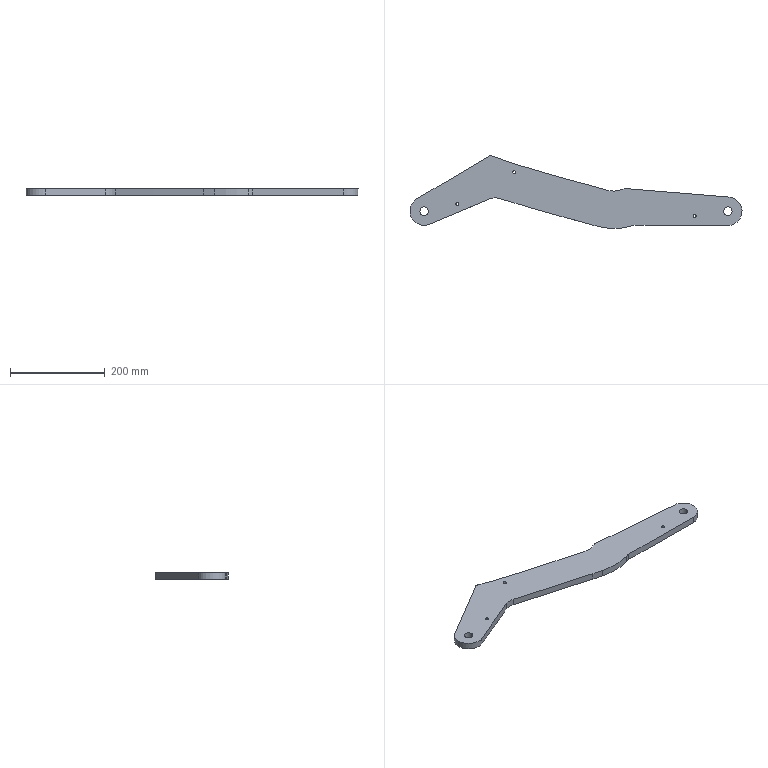NC program | NX | posted with a generic post | part box 700 x 153.975 x 14 mm
Lines 1 to 967 of 6173:
N10 G17 G21 G94 G90
(CAVITY_MILL , TOOL : D20R0)
N12 T00 M6
N14 G54
N16 G17 G0 G90 X361.565 Y64.401 S4500 M3
N18 G43 Z117. H0
N20 Z19.
N22 G94 G1 X361.412 Y64.442 Z18.994 F3500.
N24 X361.381 Y64.45 Z18.993
N26 X361.29 Y64.475 Z18.99
N28 X361.044 Y64.541 Z18.981
N30 X360.012 Y64.819 Z18.944
N32 X359.496 Y64.958 Z18.925
N34 X358.464 Y65.237 Z18.888
N36 X357.948 Y65.376 Z18.869
N38 X357.329 Y65.543 Z18.847
N40 X357.174 Y65.585 Z18.841
N42 X357.019 Y65.628 Z18.836
N44 X356.922 Y65.653 Z18.832
N46 X356.859 Y65.67 Z18.83
N48 X356.855 Y65.671
N50 X356.85 Z18.829
N52 X356.846 Y65.673
N54 X356.842 Y65.674
N56 X356.659 Y65.725 Z18.823
N58 X356.572 Y65.749 Z18.819
N60 X356.486 Y65.772 Z18.816
N62 X356.4 Y65.796 Z18.813
N64 X355.368 Y66.075 Z18.776
N66 X354.852 Y66.215 Z18.757
N68 X354.466 Y66.321 Z18.743
N70 X354.272 Y66.374 Z18.736
N72 X354.079 Y66.426 Z18.729
N74 X353.866 Y66.484 Z18.721
N76 X353.772 Y66.509 Z18.718
N78 X353.725 Y66.522 Z18.716
N80 X351.154 Y67.22 Z18.623
N82 X351.132 Y67.226
N84 X351.117 Y67.23 Z18.622
N86 X345.426 Y68.777 Z18.416
N88 X339.758 Y70.326 Z18.211
N90 X328.471 Y73.421 Z17.802
N92 X317.261 Y76.52 Z17.396
N94 X311.678 Y78.068 Z17.194
N96 X300.575 Y81.165 Z16.791
N98 X295.05 Y82.714 Z16.591
N100 X289.54 Y84.263 Z16.391
N102 X284.042 Y85.811 Z16.191
N104 X278.766 Y87.306 Z16.
N106 X273.108 Y88.909
N108 X267.673 Y90.457
N110 X262.251 Y92.006
N112 X256.852 Y93.554
N114 X251.475 Y95.103
N116 X246.109 Y96.648
N118 X240.773 Y98.171
N120 X235.47 Y99.72
N122 X229.46 Y101.483
N124 X219.734 Y104.365
N126 X213.98 Y106.087
N128 X209.427 Y107.462
N130 X203.145 Y109.375
N132 X199.3 Y110.56
N134 X194.321 Y112.108
N136 X193.857 Y112.254
N138 X189.412 Y113.657
N140 X187.666 Y114.211
N142 X181.474 Y116.211
N144 X176.83 Y117.745
N146 X173.735 Y118.785
N148 X170.627 Y119.85
N150 X169.091 Y120.382
N152 X166.204 Y121.399
N154 X164.448 Y122.029
N156 X161.936 Y122.947
N158 X159.805 Y123.74
N160 X157.815 Y124.495
N162 X155.162 Y125.531
N164 X153.891 Y126.044
N166 X152.067 Y126.791
N168 X150.187 Y127.592
N170 X148.972 Y128.117
N172 X147.426 Y128.798
N174 X146.629 Y129.213
N176 X146.618 Y129.217
N178 X145.876 Y129.432
N180 X144.329 Y129.881
N182 X144.326
N184 G3 X133.637 Y129.192 R18.085
N186 X130.388 Y127.613 R18.688
N188 G1 X-22.008 Y37.045
N190 G3 X-42.161 Y-8.75 R43.216
N192 X-4.312 Y-42.883 R43.059
N194 G1 X-4.079 Y-42.91
N196 X-4.075 Y-42.911
N198 X-2.758 Y-42.972
N200 X-1.21 Y-43.043
N202 X-1.208
N204 G3 X16.738 Y-39.674 R43.117
N206 G1 X16.798 Y-39.652
N208 X16.77 Y-39.595
N210 X16.742 Y-39.607
N212 G2 X4.084 Y-42.806 R43.
N214 X-21.987 Y36.954 R43.
N216 G1 X130.842 Y127.779
N218 G2 X147.304 Y128.786 R18.013
N220 G1 X148.863 Y128.099
N222 G3 X166.183 Y121.342 R260.503
N224 X195.387 Y111.711 R807.662
N226 X243.375 Y97.35 R2615.076
N228 X390.581 Y56.555 R6730.508
N230 X415.708 Y58.845 R36.87
N232 G1 X416.068 Y59.015
N234 G2 X425.196 Y60.668 R18.
N236 G1 X643.496 Y42.858
N238 G2 X644.084 Y-42.806 R43.
N240 X639.828 Y-43. R42.995
N242 G1 X639.792
N244 X639.789 Y-43.064
N246 X639.852 Y-43.06
N248 G3 X675.875 Y23.815 R43.064
N250 X644.312 Y42.88 R43.055
N252 G1 X644.311
N254 X642.762 Y43.007
N256 X426.043 Y60.659
N258 G3 X415.164 Y58.693 R19.291
N260 G1 X413.63 Y58.008
N262 X413.37 Y57.907
N264 X412.085 Y57.432
N266 X410.54 Y56.933
N268 X408.994 Y56.508
N270 X408.389 Y56.36
N272 X407.449 Y56.154
N274 X405.904 Y55.868
N276 X404.358 Y55.651
N278 X402.813 Y55.5
N280 X401.267 Y55.414
N282 X399.722 Y55.393
N284 X398.176 Y55.437
N286 X396.631 Y55.547
N288 X395.085 Y55.722
N290 X393.54 Y55.963
N292 X392.001 Y56.295
N294 X391.812 Y56.345
N296 X391.628 Y56.394
N298 X390.463 Y56.704
N300 X379.896 Y59.519
N302 X368.315 Y62.603
N304 X362.586 Y64.129
N306 X362.576 Y64.132
N308 X362.548 Y64.139
N310 X362.517 Y64.148
N312 X361.412 Y64.442
N314 X361.381 Y64.45
N316 X361.29 Y64.475
N318 X361.044 Y64.541
N320 X360.012 Y64.819
N322 X359.496 Y64.958
N324 X358.464 Y65.237
N326 X357.948 Y65.376
N328 X357.329 Y65.543
N330 X357.174 Y65.585
N332 X357.019 Y65.628
N334 X356.922 Y65.653
N336 X356.859 Y65.67
N338 X356.85 Y65.671
N340 X356.842 Y65.674
N342 X356.659 Y65.725
N344 X356.573 Y65.749
N346 X356.486 Y65.772
N348 X356.4 Y65.796
N350 X355.368 Y66.075
N352 X354.852 Y66.215
N354 X354.466 Y66.321
N356 X354.272 Y66.374
N358 X354.079 Y66.426
N360 X353.866 Y66.484
N362 X353.772 Y66.509
N364 X353.725 Y66.522
N366 X351.154 Y67.22
N368 X351.132 Y67.226
N370 X351.117 Y67.23
N372 X345.426 Y68.777
N374 X339.758 Y70.326
N376 X328.471 Y73.421
N378 X317.261 Y76.52
N380 X311.678 Y78.068
N382 X300.575 Y81.165
N384 X295.05 Y82.714
N386 X289.54 Y84.263
N388 X284.042 Y85.811
N390 X278.766 Y87.306
N392 Z19.
N394 G0 Z22.
N396 X361.565 Y64.401
N398 Z18.
N400 G1 X361.412 Y64.442 Z17.994
N402 X361.381 Y64.45 Z17.993
N404 X361.29 Y64.475 Z17.99
N406 X361.044 Y64.541 Z17.981
N408 X360.012 Y64.819 Z17.944
N410 X359.496 Y64.958 Z17.925
N412 X358.464 Y65.237 Z17.888
N414 X357.948 Y65.376 Z17.869
N416 X357.329 Y65.543 Z17.847
N418 X357.174 Y65.585 Z17.841
N420 X357.019 Y65.628 Z17.836
N422 X356.922 Y65.653 Z17.832
N424 X356.859 Y65.67 Z17.83
N426 X356.855 Y65.671
N428 X356.85 Z17.829
N430 X356.846 Y65.673
N432 X356.842 Y65.674
N434 X356.659 Y65.725 Z17.823
N436 X356.572 Y65.749 Z17.819
N438 X356.486 Y65.772 Z17.816
N440 X356.4 Y65.796 Z17.813
N442 X355.368 Y66.075 Z17.776
N444 X354.852 Y66.215 Z17.757
N446 X354.466 Y66.321 Z17.743
N448 X354.272 Y66.374 Z17.736
N450 X354.079 Y66.426 Z17.729
N452 X353.866 Y66.484 Z17.721
N454 X353.772 Y66.509 Z17.718
N456 X353.725 Y66.522 Z17.716
N458 X351.154 Y67.22 Z17.623
N460 X351.132 Y67.226
N462 X351.117 Y67.23 Z17.622
N464 X345.426 Y68.777 Z17.416
N466 X339.758 Y70.326 Z17.211
N468 X328.471 Y73.421 Z16.802
N470 X317.261 Y76.52 Z16.396
N472 X311.678 Y78.068 Z16.194
N474 X300.575 Y81.165 Z15.791
N476 X295.05 Y82.714 Z15.591
N478 X289.54 Y84.263 Z15.391
N480 X284.042 Y85.811 Z15.191
N482 X278.766 Y87.306 Z15.
N484 X273.108 Y88.909
N486 X267.673 Y90.457
N488 X262.251 Y92.006
N490 X256.852 Y93.554
N492 X251.475 Y95.103
N494 X246.109 Y96.648
N496 X240.773 Y98.171
N498 X235.47 Y99.72
N500 X229.46 Y101.483
N502 X219.734 Y104.365
N504 X213.98 Y106.087
N506 X209.427 Y107.462
N508 X203.145 Y109.375
N510 X199.3 Y110.56
N512 X194.321 Y112.108
N514 X193.857 Y112.254
N516 X189.412 Y113.657
N518 X187.666 Y114.211
N520 X181.474 Y116.211
N522 X176.83 Y117.745
N524 X173.735 Y118.785
N526 X170.627 Y119.85
N528 X169.091 Y120.382
N530 X166.204 Y121.399
N532 X164.448 Y122.029
N534 X161.936 Y122.947
N536 X159.805 Y123.74
N538 X157.815 Y124.495
N540 X155.162 Y125.531
N542 X153.891 Y126.044
N544 X152.067 Y126.791
N546 X150.187 Y127.592
N548 X148.972 Y128.117
N550 X147.426 Y128.798
N552 X146.629 Y129.213
N554 X146.618 Y129.217
N556 X145.876 Y129.432
N558 X144.329 Y129.881
N560 X144.326
N562 G3 X133.637 Y129.192 R18.085
N564 X130.388 Y127.613 R18.688
N566 G1 X-22.008 Y37.045
N568 G3 X-42.161 Y-8.75 R43.216
N570 X-4.312 Y-42.883 R43.059
N572 G1 X-4.079 Y-42.91
N574 X-4.075 Y-42.911
N576 X-2.758 Y-42.972
N578 X-1.21 Y-43.043
N580 X-1.208
N582 G3 X16.738 Y-39.674 R43.117
N584 G1 X16.798 Y-39.652
N586 X16.77 Y-39.595
N588 X16.742 Y-39.607
N590 G2 X4.084 Y-42.806 R43.
N592 X-21.987 Y36.954 R43.
N594 G1 X130.842 Y127.779
N596 G2 X147.304 Y128.786 R18.013
N598 G1 X148.863 Y128.099
N600 G3 X166.184 Y121.342 R260.849
N602 X195.387 Y111.711 R807.471
N604 X243.375 Y97.35 R2613.425
N606 X390.581 Y56.555 R6731.408
N608 X415.708 Y58.845 R36.87
N610 G1 X416.068 Y59.015
N612 G2 X425.196 Y60.668 R18.
N614 G1 X643.496 Y42.858
N616 G2 X644.084 Y-42.806 R43.
N618 X639.828 Y-43. R42.995
N620 G1 X639.792
N622 X639.789 Y-43.064
N624 X639.852 Y-43.06
N626 G3 X675.875 Y23.815 R43.064
N628 X644.312 Y42.88 R43.055
N630 G1 X644.311
N632 X642.762 Y43.007
N634 X426.043 Y60.659
N636 G3 X415.164 Y58.693 R19.291
N638 G1 X413.63 Y58.008
N640 X413.37 Y57.907
N642 X412.085 Y57.432
N644 X410.54 Y56.933
N646 X408.994 Y56.508
N648 X408.389 Y56.36
N650 X407.449 Y56.154
N652 X405.904 Y55.868
N654 X404.358 Y55.651
N656 X402.813 Y55.5
N658 X401.267 Y55.414
N660 X399.722 Y55.393
N662 X398.176 Y55.437
N664 X396.631 Y55.547
N666 X395.085 Y55.722
N668 X393.54 Y55.963
N670 X392.001 Y56.295
N672 X391.812 Y56.345
N674 X391.628 Y56.394
N676 X390.463 Y56.704
N678 X379.896 Y59.519
N680 X368.315 Y62.603
N682 X362.586 Y64.129
N684 X362.576 Y64.132
N686 X362.548 Y64.139
N688 X362.517 Y64.148
N690 X361.412 Y64.442
N692 X361.381 Y64.45
N694 X361.29 Y64.475
N696 X361.044 Y64.541
N698 X360.012 Y64.819
N700 X359.496 Y64.958
N702 X358.464 Y65.237
N704 X357.948 Y65.376
N706 X357.329 Y65.543
N708 X357.174 Y65.585
N710 X357.019 Y65.628
N712 X356.922 Y65.653
N714 X356.859 Y65.67
N716 X356.85 Y65.671
N718 X356.842 Y65.674
N720 X356.659 Y65.725
N722 X356.573 Y65.749
N724 X356.486 Y65.772
N726 X356.4 Y65.796
N728 X355.368 Y66.075
N730 X354.852 Y66.215
N732 X354.466 Y66.321
N734 X354.272 Y66.374
N736 X354.079 Y66.426
N738 X353.866 Y66.484
N740 X353.772 Y66.509
N742 X353.725 Y66.522
N744 X351.154 Y67.22
N746 X351.132 Y67.226
N748 X351.117 Y67.23
N750 X345.426 Y68.777
N752 X339.758 Y70.326
N754 X328.471 Y73.421
N756 X317.261 Y76.52
N758 X311.678 Y78.068
N760 X300.575 Y81.165
N762 X295.05 Y82.714
N764 X289.54 Y84.263
N766 X284.042 Y85.811
N768 X278.766 Y87.306
N770 Z18.
N772 G0 Z21.
N774 X361.565 Y64.401
N776 Z17.
N778 G1 X361.412 Y64.442 Z16.994
N780 X361.381 Y64.45 Z16.993
N782 X361.29 Y64.475 Z16.99
N784 X361.044 Y64.541 Z16.981
N786 X360.012 Y64.819 Z16.944
N788 X359.496 Y64.958 Z16.925
N790 X358.464 Y65.237 Z16.888
N792 X357.948 Y65.376 Z16.869
N794 X357.329 Y65.543 Z16.847
N796 X357.174 Y65.585 Z16.841
N798 X357.019 Y65.628 Z16.836
N800 X356.922 Y65.653 Z16.832
N802 X356.859 Y65.67 Z16.83
N804 X356.855 Y65.671
N806 X356.85 Z16.829
N808 X356.846 Y65.673
N810 X356.842 Y65.674
N812 X356.659 Y65.725 Z16.823
N814 X356.573 Y65.749 Z16.819
N816 X356.486 Y65.772 Z16.816
N818 X356.4 Y65.796 Z16.813
N820 X355.368 Y66.075 Z16.776
N822 X354.852 Y66.215 Z16.757
N824 X354.466 Y66.321 Z16.743
N826 X354.272 Y66.374 Z16.736
N828 X354.079 Y66.426 Z16.729
N830 X353.866 Y66.484 Z16.721
N832 X353.772 Y66.509 Z16.718
N834 X353.725 Y66.522 Z16.716
N836 X351.154 Y67.22 Z16.623
N838 X351.132 Y67.226
N840 X351.117 Y67.23 Z16.622
N842 X345.426 Y68.777 Z16.416
N844 X339.758 Y70.326 Z16.211
N846 X328.471 Y73.421 Z15.802
N848 X317.261 Y76.52 Z15.396
N850 X311.678 Y78.068 Z15.194
N852 X300.575 Y81.165 Z14.791
N854 X295.05 Y82.714 Z14.591
N856 X289.54 Y84.263 Z14.391
N858 X284.042 Y85.811 Z14.191
N860 X278.766 Y87.306 Z14.
N862 X273.108 Y88.909
N864 X267.673 Y90.457
N866 X262.251 Y92.006
N868 X256.852 Y93.554
N870 X251.475 Y95.103
N872 X246.109 Y96.648
N874 X240.773 Y98.171
N876 X235.47 Y99.72
N878 X229.46 Y101.483
N880 X219.734 Y104.365
N882 X213.98 Y106.087
N884 X209.427 Y107.462
N886 X203.145 Y109.375
N888 X199.3 Y110.56
N890 X194.321 Y112.108
N892 X193.857 Y112.254
N894 X189.412 Y113.657
N896 X187.666 Y114.211
N898 X181.474 Y116.211
N900 X176.83 Y117.745
N902 X173.735 Y118.785
N904 X170.627 Y119.85
N906 X169.091 Y120.382
N908 X166.204 Y121.399
N910 X164.448 Y122.029
N912 X161.936 Y122.947
N914 X159.805 Y123.74
N916 X157.815 Y124.495
N918 X155.162 Y125.531
N920 X153.891 Y126.044
N922 X152.067 Y126.791
N924 X150.187 Y127.592
N926 X148.972 Y128.117
N928 X147.426 Y128.798
N930 X146.629 Y129.213
N932 X146.618 Y129.217
N934 X145.876 Y129.432
N936 X144.329 Y129.881
N938 X144.326
N940 G3 X133.637 Y129.192 R18.085
N942 X130.388 Y127.613 R18.688
N944 G1 X-22.008 Y37.045
N946 G3 X-42.161 Y-8.75 R43.216
N948 X-4.312 Y-42.883 R43.059
N950 G1 X-4.079 Y-42.91
N952 X-4.075 Y-42.911
N954 X-2.758 Y-42.972
N956 X-1.21 Y-43.043
N958 X-1.208
N960 G3 X16.738 Y-39.674 R43.117
N962 G1 X16.798 Y-39.652
N964 X16.77 Y-39.595
N966 X16.742 Y-39.607
N968 G2 X4.084 Y-42.806 R43.
N970 X-21.987 Y36.954 R43.
N972 G1 X130.854 Y127.786
N974 G2 X147.304 Y128.786 R18.
N976 G1 X148.863 Y128.099
N978 G3 X166.184 Y121.342 R258.967
N980 X195.387 Y111.712 R808.033
N982 X243.375 Y97.351 R2611.775
N984 X390.581 Y56.555 R6717.879
N986 X415.708 Y58.845 R36.87
N988 G1 X416.068 Y59.015
N990 G2 X425.196 Y60.668 R18.
N992 G1 X643.496 Y42.858
N994 G2 X644.084 Y-42.806 R43.
N996 X639.828 Y-43. R42.995
N998 G1 X639.792
N1000 X639.789 Y-43.064
N1002 X639.852 Y-43.06
N1004 G3 X675.875 Y23.815 R43.064
N1006 X644.312 Y42.88 R43.055
N1008 G1 X644.311
N1010 X642.762 Y43.007
N1012 X426.043 Y60.659
N1014 G3 X415.164 Y58.693 R19.291
N1016 G1 X413.63 Y58.008
N1018 X413.37 Y57.907
N1020 X412.085 Y57.432
N1022 X410.54 Y56.933
N1024 X408.994 Y56.508
N1026 X408.389 Y56.36
N1028 X407.449 Y56.154
N1030 X405.904 Y55.868
N1032 X404.358 Y55.651
N1034 X402.813 Y55.5
N1036 X401.267 Y55.414
N1038 X399.722 Y55.393
N1040 X398.176 Y55.437
N1042 X396.631 Y55.547
N1044 X395.085 Y55.722
N1046 X393.54 Y55.963
N1048 X392.001 Y56.295
N1050 X391.812 Y56.345
N1052 X391.628 Y56.394
N1054 X390.463 Y56.704
N1056 X379.896 Y59.519
N1058 X368.315 Y62.603
N1060 X362.586 Y64.129
N1062 X362.576 Y64.132
N1064 X362.548 Y64.139
N1066 X362.517 Y64.148
N1068 X361.412 Y64.442
N1070 X361.381 Y64.45
N1072 X361.29 Y64.475
N1074 X361.044 Y64.541
N1076 X360.012 Y64.819
N1078 X359.496 Y64.958
N1080 X358.464 Y65.237
N1082 X357.948 Y65.376
N1084 X357.329 Y65.543
N1086 X357.174 Y65.585
N1088 X357.019 Y65.628
N1090 X356.922 Y65.653
N1092 X356.859 Y65.67
N1094 X356.85 Y65.671
N1096 X356.842 Y65.674
N1098 X356.659 Y65.725
N1100 X356.573 Y65.749
N1102 X356.486 Y65.772
N1104 X356.4 Y65.796
N1106 X355.368 Y66.075
N1108 X354.852 Y66.215
N1110 X354.466 Y66.321
N1112 X354.272 Y66.374
N1114 X354.079 Y66.426
N1116 X353.866 Y66.484
N1118 X353.772 Y66.509
N1120 X353.725 Y66.522
N1122 X351.154 Y67.22
N1124 X351.132 Y67.226
N1126 X351.117 Y67.23
N1128 X345.426 Y68.777
N1130 X339.758 Y70.326
N1132 X328.471 Y73.421
N1134 X317.261 Y76.52
N1136 X311.678 Y78.068
N1138 X300.575 Y81.165
N1140 X295.05 Y82.714
N1142 X289.54 Y84.263
N1144 X284.042 Y85.811
N1146 X278.766 Y87.306
N1148 Z17.
N1150 G0 Z20.
N1152 X361.565 Y64.401
N1154 Z16.
N1156 G1 X361.412 Y64.442 Z15.994
N1158 X361.381 Y64.45 Z15.993
N1160 X361.29 Y64.475 Z15.99
N1162 X361.044 Y64.541 Z15.981
N1164 X360.012 Y64.819 Z15.944
N1166 X359.496 Y64.958 Z15.925
N1168 X358.464 Y65.237 Z15.888
N1170 X357.948 Y65.376 Z15.869
N1172 X357.329 Y65.543 Z15.847
N1174 X357.174 Y65.585 Z15.841
N1176 X357.019 Y65.628 Z15.836
N1178 X356.922 Y65.653 Z15.832
N1180 X356.855 Y65.671 Z15.83
N1182 X356.85 Z15.829
N1184 X356.846 Y65.673
N1186 X356.842 Y65.674
N1188 X356.573 Y65.749 Z15.819
N1190 X356.486 Y65.772 Z15.816
N1192 X356.4 Y65.796 Z15.813
N1194 X355.368 Y66.075 Z15.776
N1196 X354.852 Y66.215 Z15.757
N1198 X354.466 Y66.321 Z15.743
N1200 X354.272 Y66.374 Z15.736
N1202 X354.079 Y66.426 Z15.729
N1204 X353.866 Y66.484 Z15.721
N1206 X353.772 Y66.509 Z15.718
N1208 X353.725 Y66.522 Z15.716
N1210 X351.154 Y67.22 Z15.623
N1212 X351.132 Y67.226
N1214 X351.117 Y67.23 Z15.622
N1216 X345.426 Y68.777 Z15.416
N1218 X339.758 Y70.326 Z15.211
N1220 X328.471 Y73.421 Z14.802
N1222 X317.261 Y76.52 Z14.396
N1224 X311.678 Y78.068 Z14.194
N1226 X300.575 Y81.165 Z13.791
N1228 X295.05 Y82.714 Z13.591
N1230 X289.54 Y84.263 Z13.391
N1232 X284.042 Y85.811 Z13.191
N1234 X278.766 Y87.306 Z13.
N1236 X273.108 Y88.909
N1238 X267.673 Y90.457
N1240 X262.251 Y92.006
N1242 X256.852 Y93.554
N1244 X251.475 Y95.103
N1246 X246.109 Y96.648
N1248 X240.773 Y98.171
N1250 X235.47 Y99.72
N1252 X229.46 Y101.483
N1254 X219.734 Y104.365
N1256 X213.98 Y106.087
N1258 X209.427 Y107.462
N1260 X203.145 Y109.375
N1262 X199.3 Y110.56
N1264 X194.321 Y112.108
N1266 X193.857 Y112.254
N1268 X189.412 Y113.657
N1270 X187.666 Y114.211
N1272 X181.474 Y116.211
N1274 X176.83 Y117.745
N1276 X173.735 Y118.785
N1278 X170.627 Y119.85
N1280 X169.091 Y120.382
N1282 X166.204 Y121.399
N1284 X164.448 Y122.029
N1286 X161.936 Y122.947
N1288 X159.805 Y123.74
N1290 X157.815 Y124.495
N1292 X155.162 Y125.531
N1294 X153.891 Y126.044
N1296 X152.067 Y126.791
N1298 X150.187 Y127.592
N1300 X148.972 Y128.117
N1302 X147.426 Y128.798
N1304 X146.629 Y129.213
N1306 X146.618 Y129.217
N1308 X145.876 Y129.432
N1310 X144.329 Y129.881
N1312 X144.326
N1314 G3 X133.637 Y129.192 R18.085
N1316 X130.388 Y127.613 R18.688
N1318 G1 X-22.008 Y37.045
N1320 G3 X-42.161 Y-8.75 R43.216
N1322 X-4.312 Y-42.883 R43.059
N1324 G1 X-4.079 Y-42.91
N1326 X-4.075 Y-42.911
N1328 X-2.758 Y-42.972
N1330 X-1.21 Y-43.043
N1332 X-1.208
N1334 G3 X16.738 Y-39.674 R43.117
N1336 G1 X16.798 Y-39.652
N1338 X16.77 Y-39.595
N1340 X16.742 Y-39.607
N1342 G2 X-21.987 Y36.954 R43.
N1344 G1 X130.848 Y127.782
N1346 G2 X147.313 Y128.782 R18.016
N1348 G1 X148.844 Y128.107
N1350 G3 X166.184 Y121.342 R261.014
N1352 X195.387 Y111.712 R808.033
N1354 X243.375 Y97.351 R2611.778
N1356 X390.609 Y56.548 R6717.562
N1358 X415.708 Y58.845 R36.87
N1360 G1 X416.068 Y59.015
N1362 G2 X425.218 Y60.666 R18.042
N1364 G1 X643.496 Y42.858
N1366 G2 X639.828 Y-43. R43.
N1368 G1 X639.792
N1370 X639.789 Y-43.064
N1372 X639.852 Y-43.06
N1374 G3 X675.875 Y23.815 R43.064
N1376 X644.312 Y42.88 R43.055
N1378 G1 X644.311
N1380 X642.762 Y43.007
N1382 X426.043 Y60.659
N1384 G3 X415.164 Y58.693 R19.291
N1386 G1 X413.63 Y58.008
N1388 X413.37 Y57.907
N1390 X412.085 Y57.432
N1392 X410.54 Y56.933
N1394 X408.994 Y56.508
N1396 X408.389 Y56.36
N1398 X407.449 Y56.154
N1400 X405.904 Y55.868
N1402 X404.358 Y55.651
N1404 X402.813 Y55.5
N1406 X401.267 Y55.414
N1408 X399.722 Y55.393
N1410 X398.176 Y55.437
N1412 X396.631 Y55.547
N1414 X395.085 Y55.722
N1416 X393.54 Y55.963
N1418 X392.001 Y56.295
N1420 X391.812 Y56.345
N1422 X391.628 Y56.394
N1424 X379.896 Y59.519
N1426 X368.315 Y62.603
N1428 X362.586 Y64.129
N1430 X362.576 Y64.132
N1432 X362.548 Y64.139
N1434 X362.517 Y64.148
N1436 X361.412 Y64.442
N1438 X361.381 Y64.45
N1440 X361.29 Y64.475
N1442 X361.044 Y64.541
N1444 X360.012 Y64.819
N1446 X359.496 Y64.958
N1448 X358.464 Y65.237
N1450 X357.948 Y65.376
N1452 X357.329 Y65.543
N1454 X357.174 Y65.585
N1456 X357.019 Y65.628
N1458 X356.922 Y65.653
N1460 X356.859 Y65.67
N1462 X356.85 Y65.671
N1464 X356.842 Y65.674
N1466 X356.573 Y65.749
N1468 X356.486 Y65.772
N1470 X356.4 Y65.796
N1472 X355.368 Y66.075
N1474 X354.852 Y66.215
N1476 X354.466 Y66.321
N1478 X354.272 Y66.374
N1480 X354.079 Y66.426
N1482 X353.866 Y66.484
N1484 X353.772 Y66.509
N1486 X353.725 Y66.522
N1488 X351.154 Y67.22
N1490 X351.132 Y67.226
N1492 X351.117 Y67.23
N1494 X345.426 Y68.777
N1496 X339.758 Y70.326
N1498 X328.471 Y73.421
N1500 X317.261 Y76.52
N1502 X311.678 Y78.068
N1504 X300.575 Y81.165
N1506 X295.05 Y82.714
N1508 X289.54 Y84.263
N1510 X284.042 Y85.811
N1512 X278.766 Y87.306
N1514 Z16.
N1516 G0 Z19.
N1518 X361.565 Y64.401
N1520 Z15.
N1522 G1 X361.412 Y64.442 Z14.994
N1524 X361.381 Y64.45 Z14.993
N1526 X361.29 Y64.475 Z14.99
N1528 X361.044 Y64.541 Z14.981
N1530 X360.012 Y64.819 Z14.944
N1532 X359.496 Y64.958 Z14.925
N1534 X358.464 Y65.237 Z14.888
N1536 X357.948 Y65.376 Z14.869
N1538 X357.329 Y65.543 Z14.847
N1540 X357.174 Y65.585 Z14.841
N1542 X357.019 Y65.628 Z14.836
N1544 X356.922 Y65.653 Z14.832
N1546 X356.855 Y65.671 Z14.83
N1548 X356.85 Z14.829
N1550 X356.846 Y65.673
N1552 X356.842 Y65.674
N1554 X356.573 Y65.749 Z14.819
N1556 X356.486 Y65.772 Z14.816
N1558 X356.4 Y65.796 Z14.813
N1560 X355.368 Y66.075 Z14.776
N1562 X354.852 Y66.215 Z14.757
N1564 X354.466 Y66.321 Z14.743
N1566 X354.272 Y66.374 Z14.736
N1568 X354.079 Y66.426 Z14.729
N1570 X353.866 Y66.484 Z14.721
N1572 X353.772 Y66.509 Z14.718
N1574 X353.725 Y66.522 Z14.716
N1576 X351.154 Y67.22 Z14.623
N1578 X351.132 Y67.226
N1580 X351.117 Y67.23 Z14.622
N1582 X345.426 Y68.777 Z14.416
N1584 X339.758 Y70.326 Z14.211
N1586 X328.471 Y73.421 Z13.802
N1588 X317.261 Y76.52 Z13.396
N1590 X311.678 Y78.068 Z13.194
N1592 X300.575 Y81.165 Z12.791
N1594 X295.05 Y82.714 Z12.591
N1596 X289.54 Y84.263 Z12.391
N1598 X284.042 Y85.811 Z12.191
N1600 X278.766 Y87.306 Z12.
N1602 X273.108 Y88.909
N1604 X267.673 Y90.457
N1606 X262.251 Y92.006
N1608 X256.852 Y93.554
N1610 X251.475 Y95.103
N1612 X246.109 Y96.648
N1614 X240.773 Y98.171
N1616 X235.47 Y99.72
N1618 X229.46 Y101.483
N1620 X219.734 Y104.365
N1622 X213.98 Y106.087
N1624 X209.427 Y107.462
N1626 X203.145 Y109.375
N1628 X199.3 Y110.56
N1630 X194.321 Y112.108
N1632 X193.857 Y112.254
N1634 X189.412 Y113.657
N1636 X187.666 Y114.211
N1638 X181.474 Y116.211
N1640 X176.83 Y117.745
N1642 X173.735 Y118.785
N1644 X170.627 Y119.85
N1646 X169.091 Y120.382
N1648 X166.204 Y121.399
N1650 X164.448 Y122.029
N1652 X161.936 Y122.947
N1654 X159.805 Y123.74
N1656 X157.815 Y124.495
N1658 X155.162 Y125.531
N1660 X153.891 Y126.044
N1662 X152.067 Y126.791
N1664 X150.187 Y127.592
N1666 X148.972 Y128.117
N1668 X147.426 Y128.798
N1670 X146.629 Y129.213
N1672 X146.618 Y129.217
N1674 X145.876 Y129.432
N1676 X144.329 Y129.881
N1678 X144.326
N1680 G3 X133.637 Y129.192 R18.085
N1682 X130.388 Y127.613 R18.688
N1684 G1 X-22.008 Y37.045
N1686 G3 X-42.161 Y-8.75 R43.216
N1688 X-4.312 Y-42.883 R43.059
N1690 G1 X-4.079 Y-42.91
N1692 X-4.075 Y-42.911
N1694 X-2.758 Y-42.972
N1696 X-1.21 Y-43.043
N1698 X-1.208
N1700 G3 X16.738 Y-39.674 R43.117
N1702 G1 X16.798 Y-39.652
N1704 X16.77 Y-39.595
N1706 X16.742 Y-39.607
N1708 G2 X-21.987 Y36.954 R43.
N1710 G1 X130.843 Y127.779
N1712 G2 X147.313 Y128.782 R18.022
N1714 G1 X148.844 Y128.107
N1716 G3 X166.184 Y121.342 R261.015
N1718 X195.387 Y111.712 R808.034
N1720 X243.375 Y97.351 R2611.781
N1722 X390.61 Y56.548 R6717.559
N1724 X415.708 Y58.845 R36.87
N1726 G1 X416.068 Y59.015
N1728 G2 X425.211 Y60.667 R18.029
N1730 G1 X643.496 Y42.858
N1732 G2 X639.828 Y-43. R43.
N1734 G1 X639.792
N1736 X639.789 Y-43.064
N1738 X639.852 Y-43.06
N1740 G3 X675.875 Y23.815 R43.064
N1742 X644.312 Y42.88 R43.055
N1744 G1 X644.311
N1746 X642.762 Y43.007
N1748 X426.043 Y60.659
N1750 G3 X415.164 Y58.693 R19.291
N1752 G1 X413.63 Y58.008
N1754 X413.37 Y57.907
N1756 X412.085 Y57.432
N1758 X410.54 Y56.933
N1760 X408.994 Y56.508
N1762 X408.389 Y56.36
N1764 X407.449 Y56.154
N1766 X405.904 Y55.868
N1768 X404.358 Y55.651
N1770 X402.813 Y55.5
N1772 X401.267 Y55.414
N1774 X399.722 Y55.393
N1776 X398.176 Y55.437
N1778 X396.631 Y55.547
N1780 X395.085 Y55.722
N1782 X393.54 Y55.963
N1784 X392.001 Y56.295
N1786 X391.812 Y56.345
N1788 X391.628 Y56.394
N1790 X379.896 Y59.519
N1792 X368.315 Y62.603
N1794 X362.586 Y64.129
N1796 X362.576 Y64.132
N1798 X362.548 Y64.139
N1800 X362.517 Y64.148
N1802 X361.412 Y64.442
N1804 X361.381 Y64.45
N1806 X361.29 Y64.475
N1808 X361.044 Y64.541
N1810 X360.012 Y64.819
N1812 X359.496 Y64.958
N1814 X358.464 Y65.237
N1816 X357.948 Y65.376
N1818 X357.329 Y65.543
N1820 X357.174 Y65.585
N1822 X357.019 Y65.628
N1824 X356.922 Y65.653
N1826 X356.859 Y65.67
N1828 X356.85 Y65.671
N1830 X356.842 Y65.674
N1832 X356.573 Y65.749
N1834 X356.486 Y65.772
N1836 X356.4 Y65.796
N1838 X355.368 Y66.075
N1840 X354.852 Y66.215
N1842 X354.466 Y66.321
N1844 X354.272 Y66.374
N1846 X354.079 Y66.426
N1848 X353.866 Y66.484
N1850 X353.772 Y66.509
N1852 X353.725 Y66.522
N1854 X351.154 Y67.22
N1856 X351.132 Y67.226
N1858 X351.117 Y67.23
N1860 X345.426 Y68.777
N1862 X339.758 Y70.326
N1864 X328.471 Y73.421
N1866 X317.261 Y76.52
N1868 X311.678 Y78.068
N1870 X300.575 Y81.165
N1872 X295.05 Y82.714
N1874 X289.54 Y84.263
N1876 X284.042 Y85.811
N1878 X278.766 Y87.306
N1880 Z15.
N1882 G0 Z18.
N1884 X361.565 Y64.401
N1886 Z14.
N1888 G1 X361.412 Y64.442 Z13.994
N1890 X361.381 Y64.45 Z13.993
N1892 X361.29 Y64.475 Z13.99
N1894 X361.044 Y64.541 Z13.981
N1896 X360.012 Y64.819 Z13.944
N1898 X359.496 Y64.958 Z13.925
N1900 X358.464 Y65.237 Z13.888
N1902 X357.948 Y65.376 Z13.869
N1904 X357.329 Y65.543 Z13.847
N1906 X357.174 Y65.585 Z13.841
N1908 X357.019 Y65.628 Z13.836
N1910 X356.922 Y65.653 Z13.832
N1912 X356.855 Y65.671 Z13.83
N1914 X356.85 Z13.829
N1916 X356.846 Y65.673
N1918 X356.842 Y65.674
N1920 X356.659 Y65.725 Z13.823
N1922 X356.572 Y65.749 Z13.819
N1924 X356.486 Y65.772 Z13.816
N1926 X356.4 Y65.796 Z13.813
N1928 X355.368 Y66.075 Z13.776
N1930 X354.852 Y66.215 Z13.757
N1932 X354.466 Y66.321 Z13.743